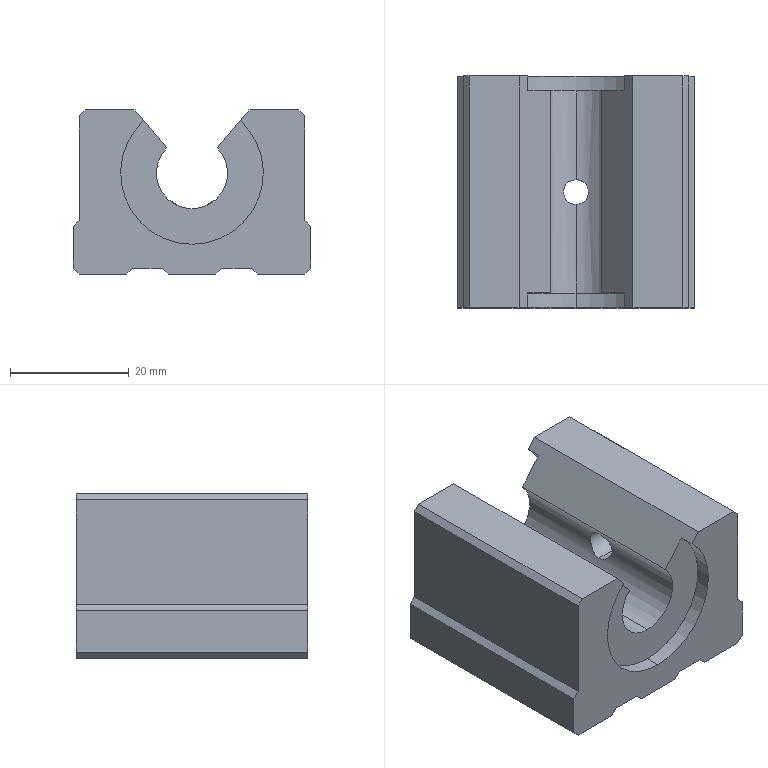Part | SolidWorks | features BaseBody 1 | 1 solid | 52 faces | box 40 x 39 x 27.6 mm | volume 31300 mm3 | plane 27 | cylinder 17 | cone 8 | commonest cylinder face diameters 4.2 x10 24 x3 5 x2 12 x2